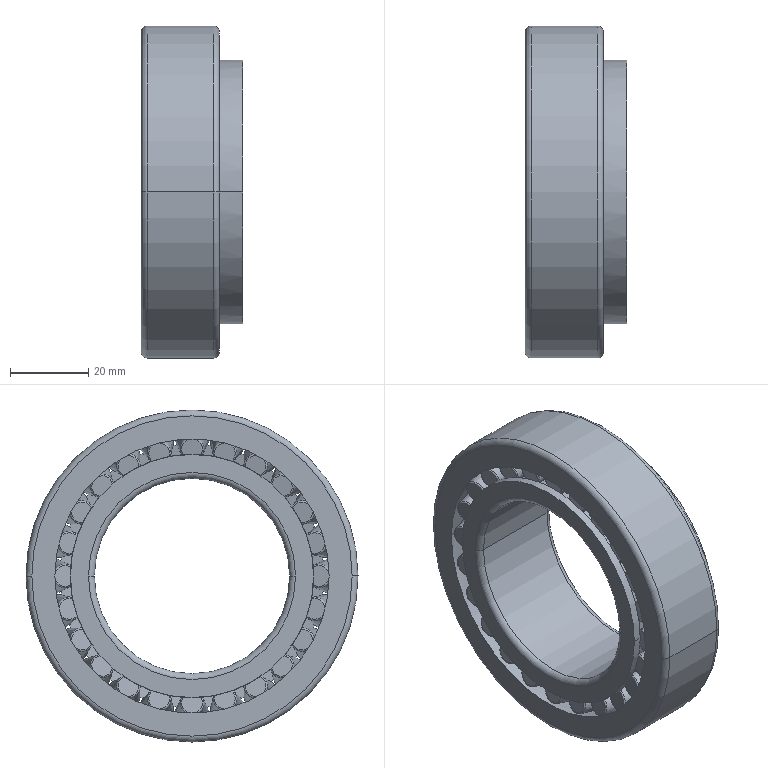Part | NX | features BREP 1 | 1 solid | 220 faces | box 26 x 85 x 85 mm | volume 69524 mm3 | torus 104 | cone 56 | plane 52 | cylinder 8 | commonest cylinder face diameters 50 x2 62.269 x2 67.5 x2 85 x2